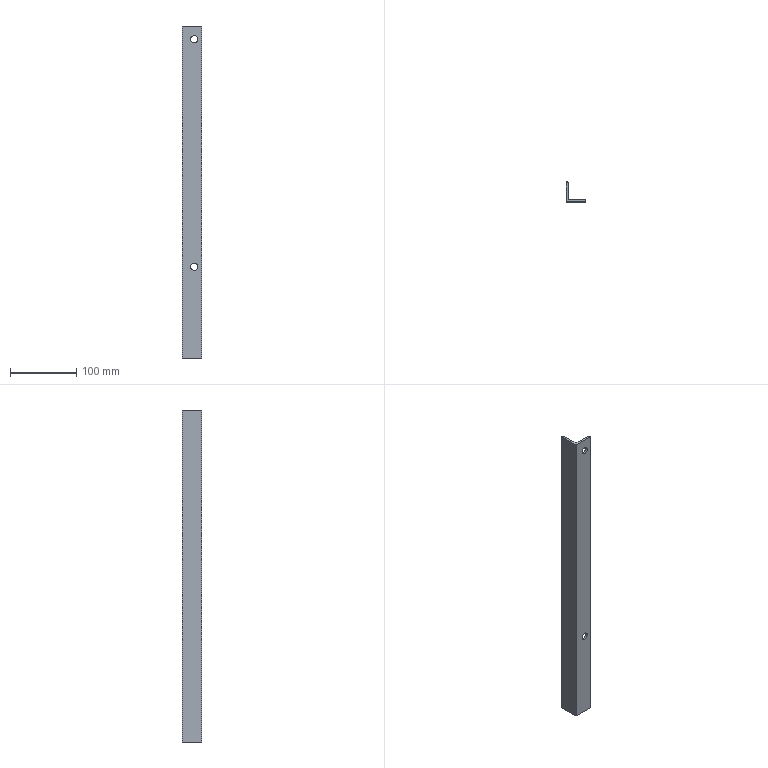Part | SolidWorks | features Extrusion 1, ICE 1, LPattern 1 | 1 solid | 15 faces | box 30 x 30 x 502 mm | volume 84841 mm3 | plane 8 | cylinder 7 | commonest cylinder face diameters 11 x4 4 x3
STEP:
#1=CARTESIAN_POINT('',(18.5,3.,143.5));
#2=VERTEX_POINT('',#1);
#3=CARTESIAN_POINT('',(18.5,3.,132.5));
#4=VERTEX_POINT('',#3);
#5=CARTESIAN_POINT('',(18.5,3.,138.));
#6=DIRECTION('',(0.,-1.,0.));
#7=DIRECTION('',(0.,0.,-1.));
#8=AXIS2_PLACEMENT_3D('',#5,#6,#7);
#9=CIRCLE('',#8,5.5);
#10=EDGE_CURVE('',#2,#4,#9,.T.);
#11=ORIENTED_EDGE('',*,*,#10,.F.);
#12=CARTESIAN_POINT('',(18.5,0.,143.5));
#13=VERTEX_POINT('',#12);
#14=CARTESIAN_POINT('',(18.5,3.,143.5));
#15=DIRECTION('',(0.,-1.,0.));
#16=VECTOR('',#15,1000.);
#17=LINE('',#14,#16);
#18=EDGE_CURVE('',#2,#13,#17,.T.);
#19=ORIENTED_EDGE('',*,*,#18,.T.);
#20=CARTESIAN_POINT('',(18.5,0.,132.5));
#21=VERTEX_POINT('',#20);
#22=CARTESIAN_POINT('',(18.5,0.,138.));
#23=DIRECTION('',(0.,-1.,0.));
#24=DIRECTION('',(0.,0.,-1.));
#25=AXIS2_PLACEMENT_3D('',#22,#23,#24);
#26=CIRCLE('',#25,5.5);
#27=EDGE_CURVE('',#13,#21,#26,.T.);
#28=ORIENTED_EDGE('',*,*,#27,.T.);
#29=CARTESIAN_POINT('',(18.5,3.,132.5));
#30=DIRECTION('',(0.,-1.,0.));
#31=VECTOR('',#30,1000.);
#32=LINE('',#29,#31);
#33=EDGE_CURVE('',#4,#21,#32,.T.);
#34=ORIENTED_EDGE('',*,*,#33,.F.);
#35=EDGE_LOOP('',(#11,#19,#28,#34));
#36=FACE_OUTER_BOUND('',#35,.T.);
#37=CARTESIAN_POINT('',(18.5,3.,138.));
#38=DIRECTION('',(0.,-1.,0.));
#39=DIRECTION('',(0.,0.,-1.));
#40=AXIS2_PLACEMENT_3D('',#37,#38,#39);
#41=CYLINDRICAL_SURFACE('',#40,5.5);
#42=ADVANCED_FACE('',(#36),#41,.F.);
#43=CARTESIAN_POINT('',(18.5,3.,487.5));
#44=VERTEX_POINT('',#43);
#45=CARTESIAN_POINT('',(18.5,3.,476.5));
#46=VERTEX_POINT('',#45);
#47=CARTESIAN_POINT('',(18.5,3.,482.));
#48=DIRECTION('',(0.,-1.,0.));
#49=DIRECTION('',(0.,0.,-1.));
#50=AXIS2_PLACEMENT_3D('',#47,#48,#49);
#51=CIRCLE('',#50,5.5);
#52=EDGE_CURVE('',#44,#46,#51,.T.);
#53=ORIENTED_EDGE('',*,*,#52,.F.);
#54=CARTESIAN_POINT('',(18.5,0.,487.5));
#55=VERTEX_POINT('',#54);
#56=CARTESIAN_POINT('',(18.5,3.,487.5));
#57=DIRECTION('',(0.,-1.,0.));
#58=VECTOR('',#57,1000.);
#59=LINE('',#56,#58);
#60=EDGE_CURVE('',#44,#55,#59,.T.);
#61=ORIENTED_EDGE('',*,*,#60,.T.);
#62=CARTESIAN_POINT('',(18.5,0.,476.5));
#63=VERTEX_POINT('',#62);
#64=CARTESIAN_POINT('',(18.5,0.,482.));
#65=DIRECTION('',(0.,-1.,0.));
#66=DIRECTION('',(0.,0.,-1.));
#67=AXIS2_PLACEMENT_3D('',#64,#65,#66);
#68=CIRCLE('',#67,5.5);
#69=EDGE_CURVE('',#55,#63,#68,.T.);
#70=ORIENTED_EDGE('',*,*,#69,.T.);
#71=CARTESIAN_POINT('',(18.5,3.,476.5));
#72=DIRECTION('',(0.,-1.,0.));
#73=VECTOR('',#72,1000.);
#74=LINE('',#71,#73);
#75=EDGE_CURVE('',#46,#63,#74,.T.);
#76=ORIENTED_EDGE('',*,*,#75,.F.);
#77=EDGE_LOOP('',(#53,#61,#70,#76));
#78=FACE_OUTER_BOUND('',#77,.T.);
#79=CARTESIAN_POINT('',(18.5,3.,482.));
#80=DIRECTION('',(0.,-1.,0.));
#81=DIRECTION('',(0.,0.,-1.));
#82=AXIS2_PLACEMENT_3D('',#79,#80,#81);
#83=CYLINDRICAL_SURFACE('',#82,5.5);
#84=ADVANCED_FACE('',(#78),#83,.F.);
#85=CARTESIAN_POINT('',(0.,30.,0.));
#86=VERTEX_POINT('',#85);
#87=CARTESIAN_POINT('',(0.,0.,0.));
#88=VERTEX_POINT('',#87);
#89=CARTESIAN_POINT('',(0.,0.,0.));
#90=DIRECTION('',(0.,-1.,0.));
#91=VECTOR('',#90,1000.);
#92=LINE('',#89,#91);
#93=EDGE_CURVE('',#86,#88,#92,.T.);
#94=ORIENTED_EDGE('',*,*,#93,.T.);
#95=CARTESIAN_POINT('',(0.,0.,502.));
#96=VERTEX_POINT('',#95);
#97=CARTESIAN_POINT('',(0.,0.,502.));
#98=DIRECTION('',(0.,0.,-1.));
#99=VECTOR('',#98,1000.);
#100=LINE('',#97,#99);
#101=EDGE_CURVE('',#96,#88,#100,.T.);
#102=ORIENTED_EDGE('',*,*,#101,.F.);
#103=CARTESIAN_POINT('',(0.,30.,502.));
#104=VERTEX_POINT('',#103);
#105=CARTESIAN_POINT('',(0.,0.,502.));
#106=DIRECTION('',(0.,-1.,0.));
#107=VECTOR('',#106,1000.);
#108=LINE('',#105,#107);
#109=EDGE_CURVE('',#104,#96,#108,.T.);
#110=ORIENTED_EDGE('',*,*,#109,.F.);
#111=CARTESIAN_POINT('',(0.,30.,502.));
#112=DIRECTION('',(0.,0.,-1.));
#113=VECTOR('',#112,1000.);
#114=LINE('',#111,#113);
#115=EDGE_CURVE('',#104,#86,#114,.T.);
#116=ORIENTED_EDGE('',*,*,#115,.T.);
#117=EDGE_LOOP('',(#94,#102,#110,#116));
#118=FACE_OUTER_BOUND('',#117,.T.);
#119=CARTESIAN_POINT('',(0.,0.,502.));
#120=DIRECTION('',(1.,0.,0.));
#121=DIRECTION('',(0.,0.,-1.));
#122=AXIS2_PLACEMENT_3D('',#119,#120,#121);
#123=PLANE('',#122);
#124=ADVANCED_FACE('',(#118),#123,.F.);
#125=CARTESIAN_POINT('',(18.5,0.,138.));
#126=DIRECTION('',(0.,-1.,0.));
#127=DIRECTION('',(0.,0.,-1.));
#128=AXIS2_PLACEMENT_3D('',#125,#126,#127);
#129=CIRCLE('',#128,5.5);
#130=EDGE_CURVE('',#21,#13,#129,.T.);
#131=ORIENTED_EDGE('',*,*,#130,.F.);
#132=ORIENTED_EDGE('',*,*,#27,.F.);
#133=EDGE_LOOP('',(#131,#132));
#134=FACE_BOUND('',#133,.T.);
#135=CARTESIAN_POINT('',(18.5,0.,482.));
#136=DIRECTION('',(0.,-1.,0.));
#137=DIRECTION('',(0.,0.,-1.));
#138=AXIS2_PLACEMENT_3D('',#135,#136,#137);
#139=CIRCLE('',#138,5.5);
#140=EDGE_CURVE('',#63,#55,#139,.T.);
#141=ORIENTED_EDGE('',*,*,#140,.F.);
#142=ORIENTED_EDGE('',*,*,#69,.F.);
#143=EDGE_LOOP('',(#141,#142));
#144=FACE_BOUND('',#143,.T.);
#145=CARTESIAN_POINT('',(30.,0.,0.));
#146=VERTEX_POINT('',#145);
#147=CARTESIAN_POINT('',(0.,0.,0.));
#148=DIRECTION('',(1.,0.,0.));
#149=VECTOR('',#148,1000.);
#150=LINE('',#147,#149);
#151=EDGE_CURVE('',#88,#146,#150,.T.);
#152=ORIENTED_EDGE('',*,*,#151,.T.);
#153=CARTESIAN_POINT('',(30.,0.,502.));
#154=VERTEX_POINT('',#153);
#155=CARTESIAN_POINT('',(30.,0.,502.));
#156=DIRECTION('',(0.,0.,-1.));
#157=VECTOR('',#156,1000.);
#158=LINE('',#155,#157);
#159=EDGE_CURVE('',#154,#146,#158,.T.);
#160=ORIENTED_EDGE('',*,*,#159,.F.);
#161=CARTESIAN_POINT('',(0.,0.,502.));
#162=DIRECTION('',(1.,0.,0.));
#163=VECTOR('',#162,1000.);
#164=LINE('',#161,#163);
#165=EDGE_CURVE('',#96,#154,#164,.T.);
#166=ORIENTED_EDGE('',*,*,#165,.F.);
#167=ORIENTED_EDGE('',*,*,#101,.T.);
#168=EDGE_LOOP('',(#152,#160,#166,#167));
#169=FACE_OUTER_BOUND('',#168,.T.);
#170=CARTESIAN_POINT('',(0.,0.,502.));
#171=DIRECTION('',(0.,1.,0.));
#172=DIRECTION('',(0.,0.,1.));
#173=AXIS2_PLACEMENT_3D('',#170,#171,#172);
#174=PLANE('',#173);
#175=ADVANCED_FACE('',(#134,#144,#169),#174,.F.);
#176=CARTESIAN_POINT('',(30.,1.,0.));
#177=VERTEX_POINT('',#176);
#178=CARTESIAN_POINT('',(30.,1.,0.));
#179=DIRECTION('',(0.,1.,0.));
#180=VECTOR('',#179,1000.);
#181=LINE('',#178,#180);
#182=EDGE_CURVE('',#146,#177,#181,.T.);
#183=ORIENTED_EDGE('',*,*,#182,.T.);
#184=CARTESIAN_POINT('',(30.,1.,502.));
#185=VERTEX_POINT('',#184);
#186=CARTESIAN_POINT('',(30.,1.,502.));
#187=DIRECTION('',(0.,0.,-1.));
#188=VECTOR('',#187,1000.);
#189=LINE('',#186,#188);
#190=EDGE_CURVE('',#185,#177,#189,.T.);
#191=ORIENTED_EDGE('',*,*,#190,.F.);
#192=CARTESIAN_POINT('',(30.,1.,502.));
#193=DIRECTION('',(0.,1.,0.));
#194=VECTOR('',#193,1000.);
#195=LINE('',#192,#194);
#196=EDGE_CURVE('',#154,#185,#195,.T.);
#197=ORIENTED_EDGE('',*,*,#196,.F.);
#198=ORIENTED_EDGE('',*,*,#159,.T.);
#199=EDGE_LOOP('',(#183,#191,#197,#198));
#200=FACE_OUTER_BOUND('',#199,.T.);
#201=CARTESIAN_POINT('',(30.,1.,502.));
#202=DIRECTION('',(-1.,0.,0.));
#203=DIRECTION('',(0.,0.,1.));
#204=AXIS2_PLACEMENT_3D('',#201,#202,#203);
#205=PLANE('',#204);
#206=ADVANCED_FACE('',(#200),#205,.F.);
#207=CARTESIAN_POINT('',(28.,3.,0.));
#208=VERTEX_POINT('',#207);
#209=CARTESIAN_POINT('',(28.,1.,0.));
#210=DIRECTION('',(0.,0.,1.));
#211=DIRECTION('',(1.,0.,0.));
#212=AXIS2_PLACEMENT_3D('',#209,#210,#211);
#213=CIRCLE('',#212,2.);
#214=EDGE_CURVE('',#177,#208,#213,.T.);
#215=ORIENTED_EDGE('',*,*,#214,.T.);
#216=CARTESIAN_POINT('',(28.,3.,502.));
#217=VERTEX_POINT('',#216);
#218=CARTESIAN_POINT('',(28.,3.,502.));
#219=DIRECTION('',(0.,0.,-1.));
#220=VECTOR('',#219,1000.);
#221=LINE('',#218,#220);
#222=EDGE_CURVE('',#217,#208,#221,.T.);
#223=ORIENTED_EDGE('',*,*,#222,.F.);
#224=CARTESIAN_POINT('',(28.,1.,502.));
#225=DIRECTION('',(0.,0.,1.));
#226=DIRECTION('',(1.,0.,0.));
#227=AXIS2_PLACEMENT_3D('',#224,#225,#226);
#228=CIRCLE('',#227,2.);
#229=EDGE_CURVE('',#185,#217,#228,.T.);
#230=ORIENTED_EDGE('',*,*,#229,.F.);
#231=ORIENTED_EDGE('',*,*,#190,.T.);
#232=EDGE_LOOP('',(#215,#223,#230,#231));
#233=FACE_OUTER_BOUND('',#232,.T.);
#234=CARTESIAN_POINT('',(28.,1.,502.));
#235=DIRECTION('',(0.,0.,-1.));
#236=DIRECTION('',(-1.,0.,0.));
#237=AXIS2_PLACEMENT_3D('',#234,#235,#236);
#238=CYLINDRICAL_SURFACE('',#237,2.);
#239=ADVANCED_FACE('',(#233),#238,.T.);
#240=CARTESIAN_POINT('',(18.5,3.,138.));
#241=DIRECTION('',(0.,-1.,0.));
#242=DIRECTION('',(0.,0.,-1.));
#243=AXIS2_PLACEMENT_3D('',#240,#241,#242);
#244=CIRCLE('',#243,5.5);
#245=EDGE_CURVE('',#4,#2,#244,.T.);
#246=ORIENTED_EDGE('',*,*,#245,.T.);
#247=ORIENTED_EDGE('',*,*,#10,.T.);
#248=EDGE_LOOP('',(#246,#247));
#249=FACE_BOUND('',#248,.T.);
#250=CARTESIAN_POINT('',(18.5,3.,482.));
#251=DIRECTION('',(0.,-1.,0.));
#252=DIRECTION('',(0.,0.,-1.));
#253=AXIS2_PLACEMENT_3D('',#250,#251,#252);
#254=CIRCLE('',#253,5.5);
#255=EDGE_CURVE('',#46,#44,#254,.T.);
#256=ORIENTED_EDGE('',*,*,#255,.T.);
#257=ORIENTED_EDGE('',*,*,#52,.T.);
#258=EDGE_LOOP('',(#256,#257));
#259=FACE_BOUND('',#258,.T.);
#260=CARTESIAN_POINT('',(5.,3.,0.));
#261=VERTEX_POINT('',#260);
#262=CARTESIAN_POINT('',(5.,3.,0.));
#263=DIRECTION('',(-1.,0.,0.));
#264=VECTOR('',#263,1000.);
#265=LINE('',#262,#264);
#266=EDGE_CURVE('',#208,#261,#265,.T.);
#267=ORIENTED_EDGE('',*,*,#266,.T.);
#268=CARTESIAN_POINT('',(5.,3.,502.));
#269=VERTEX_POINT('',#268);
#270=CARTESIAN_POINT('',(5.,3.,502.));
#271=DIRECTION('',(0.,0.,-1.));
#272=VECTOR('',#271,1000.);
#273=LINE('',#270,#272);
#274=EDGE_CURVE('',#269,#261,#273,.T.);
#275=ORIENTED_EDGE('',*,*,#274,.F.);
#276=CARTESIAN_POINT('',(5.,3.,502.));
#277=DIRECTION('',(-1.,0.,0.));
#278=VECTOR('',#277,1000.);
#279=LINE('',#276,#278);
#280=EDGE_CURVE('',#217,#269,#279,.T.);
#281=ORIENTED_EDGE('',*,*,#280,.F.);
#282=ORIENTED_EDGE('',*,*,#222,.T.);
#283=EDGE_LOOP('',(#267,#275,#281,#282));
#284=FACE_OUTER_BOUND('',#283,.T.);
#285=CARTESIAN_POINT('',(5.,3.,502.));
#286=DIRECTION('',(0.,-1.,0.));
#287=DIRECTION('',(0.,0.,-1.));
#288=AXIS2_PLACEMENT_3D('',#285,#286,#287);
#289=PLANE('',#288);
#290=ADVANCED_FACE('',(#249,#259,#284),#289,.F.);
#291=CARTESIAN_POINT('',(3.,5.,0.));
#292=VERTEX_POINT('',#291);
#293=CARTESIAN_POINT('',(5.,5.,0.));
#294=DIRECTION('',(0.,0.,-1.));
#295=DIRECTION('',(-1.,0.,0.));
#296=AXIS2_PLACEMENT_3D('',#293,#294,#295);
#297=CIRCLE('',#296,2.);
#298=EDGE_CURVE('',#261,#292,#297,.T.);
#299=ORIENTED_EDGE('',*,*,#298,.T.);
#300=CARTESIAN_POINT('',(3.,5.,502.));
#301=VERTEX_POINT('',#300);
#302=CARTESIAN_POINT('',(3.,5.,502.));
#303=DIRECTION('',(0.,0.,-1.));
#304=VECTOR('',#303,1000.);
#305=LINE('',#302,#304);
#306=EDGE_CURVE('',#301,#292,#305,.T.);
#307=ORIENTED_EDGE('',*,*,#306,.F.);
#308=CARTESIAN_POINT('',(5.,5.,502.));
#309=DIRECTION('',(0.,0.,-1.));
#310=DIRECTION('',(-1.,0.,0.));
#311=AXIS2_PLACEMENT_3D('',#308,#309,#310);
#312=CIRCLE('',#311,2.);
#313=EDGE_CURVE('',#269,#301,#312,.T.);
#314=ORIENTED_EDGE('',*,*,#313,.F.);
#315=ORIENTED_EDGE('',*,*,#274,.T.);
#316=EDGE_LOOP('',(#299,#307,#314,#315));
#317=FACE_OUTER_BOUND('',#316,.T.);
#318=CARTESIAN_POINT('',(5.,5.,502.));
#319=DIRECTION('',(0.,0.,-1.));
#320=DIRECTION('',(-1.,0.,0.));
#321=AXIS2_PLACEMENT_3D('',#318,#319,#320);
#322=CYLINDRICAL_SURFACE('',#321,2.);
#323=ADVANCED_FACE('',(#317),#322,.F.);
#324=CARTESIAN_POINT('',(3.,28.,0.));
#325=VERTEX_POINT('',#324);
#326=CARTESIAN_POINT('',(3.,5.,0.));
#327=DIRECTION('',(0.,1.,0.));
#328=VECTOR('',#327,1000.);
#329=LINE('',#326,#328);
#330=EDGE_CURVE('',#292,#325,#329,.T.);
#331=ORIENTED_EDGE('',*,*,#330,.T.);
#332=CARTESIAN_POINT('',(3.,28.,502.));
#333=VERTEX_POINT('',#332);
#334=CARTESIAN_POINT('',(3.,28.,502.));
#335=DIRECTION('',(0.,0.,-1.));
#336=VECTOR('',#335,1000.);
#337=LINE('',#334,#336);
#338=EDGE_CURVE('',#333,#325,#337,.T.);
#339=ORIENTED_EDGE('',*,*,#338,.F.);
#340=CARTESIAN_POINT('',(3.,5.,502.));
#341=DIRECTION('',(0.,1.,0.));
#342=VECTOR('',#341,1000.);
#343=LINE('',#340,#342);
#344=EDGE_CURVE('',#301,#333,#343,.T.);
#345=ORIENTED_EDGE('',*,*,#344,.F.);
#346=ORIENTED_EDGE('',*,*,#306,.T.);
#347=EDGE_LOOP('',(#331,#339,#345,#346));
#348=FACE_OUTER_BOUND('',#347,.T.);
#349=CARTESIAN_POINT('',(3.,5.,502.));
#350=DIRECTION('',(-1.,0.,0.));
#351=DIRECTION('',(0.,0.,1.));
#352=AXIS2_PLACEMENT_3D('',#349,#350,#351);
#353=PLANE('',#352);
#354=ADVANCED_FACE('',(#348),#353,.F.);
#355=CARTESIAN_POINT('',(1.,30.,0.));
#356=VERTEX_POINT('',#355);
#357=CARTESIAN_POINT('',(1.,28.,0.));
#358=DIRECTION('',(0.,0.,1.));
#359=DIRECTION('',(-1.,0.,0.));
#360=AXIS2_PLACEMENT_3D('',#357,#358,#359);
#361=CIRCLE('',#360,2.);
#362=EDGE_CURVE('',#325,#356,#361,.T.);
#363=ORIENTED_EDGE('',*,*,#362,.T.);
#364=CARTESIAN_POINT('',(1.,30.,502.));
#365=VERTEX_POINT('',#364);
#366=CARTESIAN_POINT('',(1.,30.,502.));
#367=DIRECTION('',(0.,0.,-1.));
#368=VECTOR('',#367,1000.);
#369=LINE('',#366,#368);
#370=EDGE_CURVE('',#365,#356,#369,.T.);
#371=ORIENTED_EDGE('',*,*,#370,.F.);
#372=CARTESIAN_POINT('',(1.,28.,502.));
#373=DIRECTION('',(0.,0.,1.));
#374=DIRECTION('',(-1.,0.,0.));
#375=AXIS2_PLACEMENT_3D('',#372,#373,#374);
#376=CIRCLE('',#375,2.);
#377=EDGE_CURVE('',#333,#365,#376,.T.);
#378=ORIENTED_EDGE('',*,*,#377,.F.);
#379=ORIENTED_EDGE('',*,*,#338,.T.);
#380=EDGE_LOOP('',(#363,#371,#378,#379));
#381=FACE_OUTER_BOUND('',#380,.T.);
#382=CARTESIAN_POINT('',(1.,28.,502.));
#383=DIRECTION('',(0.,0.,-1.));
#384=DIRECTION('',(-1.,0.,0.));
#385=AXIS2_PLACEMENT_3D('',#382,#383,#384);
#386=CYLINDRICAL_SURFACE('',#385,2.);
#387=ADVANCED_FACE('',(#381),#386,.T.);
#388=CARTESIAN_POINT('',(0.,30.,0.));
#389=DIRECTION('',(-1.,0.,0.));
#390=VECTOR('',#389,1000.);
#391=LINE('',#388,#390);
#392=EDGE_CURVE('',#356,#86,#391,.T.);
#393=ORIENTED_EDGE('',*,*,#392,.T.);
#394=ORIENTED_EDGE('',*,*,#115,.F.);
#395=CARTESIAN_POINT('',(0.,30.,502.));
#396=DIRECTION('',(-1.,0.,0.));
#397=VECTOR('',#396,1000.);
#398=LINE('',#395,#397);
#399=EDGE_CURVE('',#365,#104,#398,.T.);
#400=ORIENTED_EDGE('',*,*,#399,.F.);
#401=ORIENTED_EDGE('',*,*,#370,.T.);
#402=EDGE_LOOP('',(#393,#394,#400,#401));
#403=FACE_OUTER_BOUND('',#402,.T.);
#404=CARTESIAN_POINT('',(0.,30.,502.));
#405=DIRECTION('',(0.,-1.,0.));
#406=DIRECTION('',(0.,0.,-1.));
#407=AXIS2_PLACEMENT_3D('',#404,#405,#406);
#408=PLANE('',#407);
#409=ADVANCED_FACE('',(#403),#408,.F.);
#410=ORIENTED_EDGE('',*,*,#109,.T.);
#411=ORIENTED_EDGE('',*,*,#165,.T.);
#412=ORIENTED_EDGE('',*,*,#196,.T.);
#413=ORIENTED_EDGE('',*,*,#229,.T.);
#414=ORIENTED_EDGE('',*,*,#280,.T.);
#415=ORIENTED_EDGE('',*,*,#313,.T.);
#416=ORIENTED_EDGE('',*,*,#344,.T.);
#417=ORIENTED_EDGE('',*,*,#377,.T.);
#418=ORIENTED_EDGE('',*,*,#399,.T.);
#419=EDGE_LOOP('',(#410,#411,#412,#413,#414,#415,#416,#417,#418));
#420=FACE_OUTER_BOUND('',#419,.T.);
#421=CARTESIAN_POINT('',(1.,28.,502.));
#422=DIRECTION('',(0.,0.,-1.));
#423=DIRECTION('',(-1.,0.,0.));
#424=AXIS2_PLACEMENT_3D('',#421,#422,#423);
#425=PLANE('',#424);
#426=ADVANCED_FACE('',(#420),#425,.F.);
#427=ORIENTED_EDGE('',*,*,#93,.F.);
#428=ORIENTED_EDGE('',*,*,#392,.F.);
#429=ORIENTED_EDGE('',*,*,#362,.F.);
#430=ORIENTED_EDGE('',*,*,#330,.F.);
#431=ORIENTED_EDGE('',*,*,#298,.F.);
#432=ORIENTED_EDGE('',*,*,#266,.F.);
#433=ORIENTED_EDGE('',*,*,#214,.F.);
#434=ORIENTED_EDGE('',*,*,#182,.F.);
#435=ORIENTED_EDGE('',*,*,#151,.F.);
#436=EDGE_LOOP('',(#427,#428,#429,#430,#431,#432,#433,#434,#435));
#437=FACE_OUTER_BOUND('',#436,.T.);
#438=CARTESIAN_POINT('',(1.,28.,0.));
#439=DIRECTION('',(0.,0.,-1.));
#440=DIRECTION('',(-1.,0.,0.));
#441=AXIS2_PLACEMENT_3D('',#438,#439,#440);
#442=PLANE('',#441);
#443=ADVANCED_FACE('',(#437),#442,.T.);
#444=ORIENTED_EDGE('',*,*,#60,.F.);
#445=ORIENTED_EDGE('',*,*,#255,.F.);
#446=ORIENTED_EDGE('',*,*,#75,.T.);
#447=ORIENTED_EDGE('',*,*,#140,.T.);
#448=EDGE_LOOP('',(#444,#445,#446,#447));
#449=FACE_OUTER_BOUND('',#448,.T.);
#450=CARTESIAN_POINT('',(18.5,3.,482.));
#451=DIRECTION('',(0.,-1.,0.));
#452=DIRECTION('',(0.,0.,-1.));
#453=AXIS2_PLACEMENT_3D('',#450,#451,#452);
#454=CYLINDRICAL_SURFACE('',#453,5.5);
#455=ADVANCED_FACE('',(#449),#454,.F.);
#456=ORIENTED_EDGE('',*,*,#18,.F.);
#457=ORIENTED_EDGE('',*,*,#245,.F.);
#458=ORIENTED_EDGE('',*,*,#33,.T.);
#459=ORIENTED_EDGE('',*,*,#130,.T.);
#460=EDGE_LOOP('',(#456,#457,#458,#459));
#461=FACE_OUTER_BOUND('',#460,.T.);
#462=CARTESIAN_POINT('',(18.5,3.,138.));
#463=DIRECTION('',(0.,-1.,0.));
#464=DIRECTION('',(0.,0.,-1.));
#465=AXIS2_PLACEMENT_3D('',#462,#463,#464);
#466=CYLINDRICAL_SURFACE('',#465,5.5);
#467=ADVANCED_FACE('',(#461),#466,.F.);
#468=CLOSED_SHELL('',(#42,#84,#124,#175,#206,#239,#290,#323,#354,#387,#409,#426,#443,#455,#467));
#469=MANIFOLD_SOLID_BREP('',#468);
#470=CARTESIAN_POINT('',(0.,0.,0.));
#471=DIRECTION('',(0.,0.,1.));
#472=DIRECTION('',(1.,0.,0.));
#473=AXIS2_PLACEMENT_3D('',#470,#471,#472);
#474=(LENGTH_UNIT()NAMED_UNIT(*)SI_UNIT(.MILLI.,.METRE.));
#475=UNCERTAINTY_MEASURE_WITH_UNIT(LENGTH_MEASURE(0.00001),#474,'','');
#476=(NAMED_UNIT(*)PLANE_ANGLE_UNIT()SI_UNIT($,.RADIAN.));
#477=(NAMED_UNIT(*)SI_UNIT($,.STERADIAN.)SOLID_ANGLE_UNIT());
#478=(GEOMETRIC_REPRESENTATION_CONTEXT(3)GLOBAL_UNCERTAINTY_ASSIGNED_CONTEXT((#475))GLOBAL_UNIT_ASSIGNED_CONTEXT((#474,#476,#477))REPRESENTATION_CONTEXT('',''));
#479=ADVANCED_BREP_SHAPE_REPRESENTATION('',(#469,#473),#478);